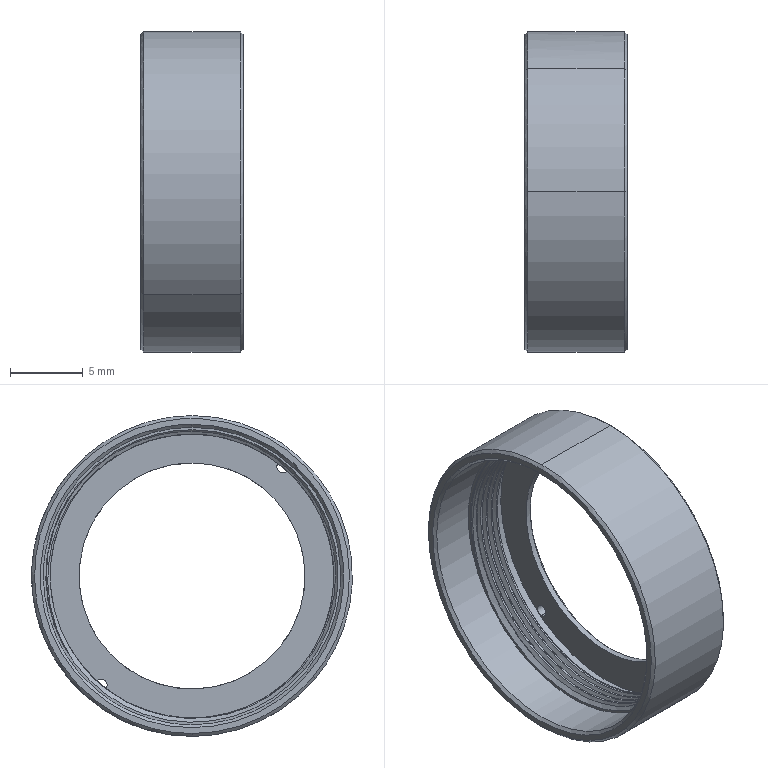Part | SolidWorks | features BaseBody 1 | 1 solid | 60 faces | box 7 x 22 x 22 mm | volume 502.064 mm3 | cylinder 32 | cone 15 | spline 8 | plane 5 | commonest cylinder face diameters 19.46 x14 0.8 x6 20.4 x6 15.5 x3 22 x3